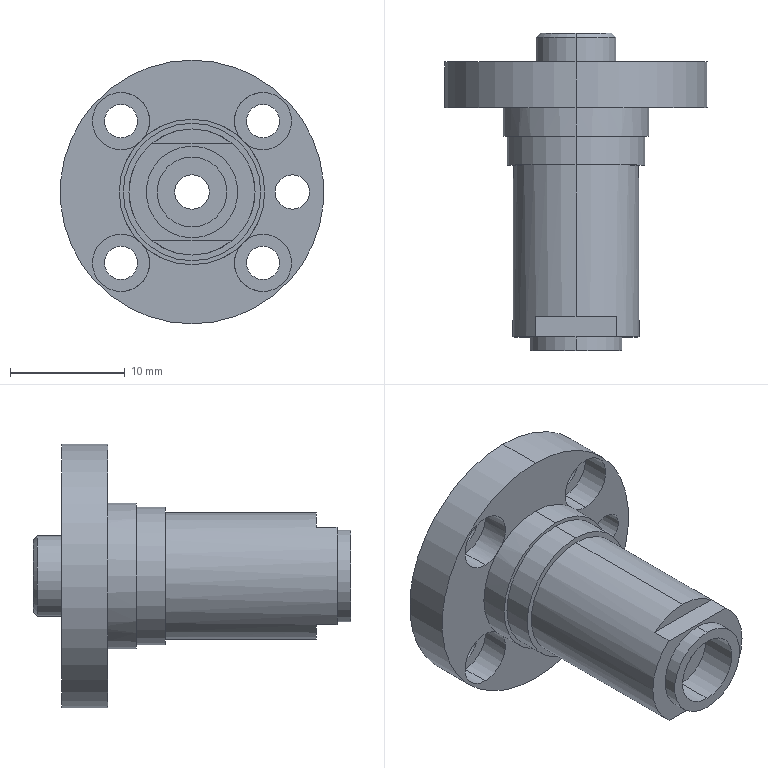Part | STEP file | 1 solid | 66 faces | box 23 x 27.7 x 23 mm | volume 2922 mm3 | cylinder 40 | plane 22 | cone 2 | torus 2 | commonest cylinder face diameters 5 x10 2.9 x8 3 x4 6.1 x2 7 x2 8 x2